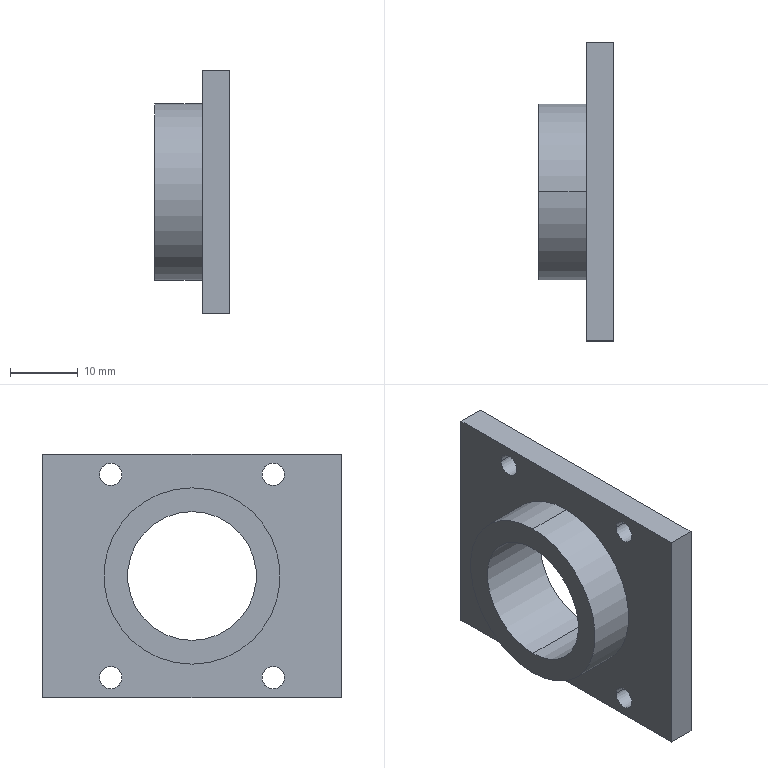Part | SolidWorks | features BaseBody 1 | 1 solid | 19 faces | box 11 x 44 x 36 mm | volume 6797 mm3 | cylinder 12 | plane 7 | commonest cylinder face diameters 3.3 x8 19 x2 26 x2
STEP:
#1=CARTESIAN_POINT('',(-2.,-13.65,33.));
#2=VERTEX_POINT('',#1);
#3=CARTESIAN_POINT('',(-2.,-10.35,33.));
#4=VERTEX_POINT('',#3);
#5=CARTESIAN_POINT('',(-2.,-12.,33.));
#6=DIRECTION('',(1.,0.,0.));
#7=DIRECTION('',(0.,1.,0.));
#8=AXIS2_PLACEMENT_3D('',#5,#6,#7);
#9=CIRCLE('',#8,1.65);
#10=EDGE_CURVE('',#2,#4,#9,.T.);
#11=ORIENTED_EDGE('',*,*,#10,.F.);
#12=CARTESIAN_POINT('',(2.,-13.65,33.));
#13=VERTEX_POINT('',#12);
#14=CARTESIAN_POINT('',(-14.2,-13.65,33.));
#15=DIRECTION('',(1.,0.,0.));
#16=VECTOR('',#15,1000.);
#17=LINE('',#14,#16);
#18=EDGE_CURVE('',#2,#13,#17,.T.);
#19=ORIENTED_EDGE('',*,*,#18,.T.);
#20=CARTESIAN_POINT('',(2.,-10.35,33.));
#21=VERTEX_POINT('',#20);
#22=CARTESIAN_POINT('',(2.,-12.,33.));
#23=DIRECTION('',(-1.,0.,0.));
#24=DIRECTION('',(0.,1.,0.));
#25=AXIS2_PLACEMENT_3D('',#22,#23,#24);
#26=CIRCLE('',#25,1.65);
#27=EDGE_CURVE('',#21,#13,#26,.T.);
#28=ORIENTED_EDGE('',*,*,#27,.F.);
#29=CARTESIAN_POINT('',(-14.2,-10.35,33.));
#30=DIRECTION('',(1.,0.,0.));
#31=VECTOR('',#30,1000.);
#32=LINE('',#29,#31);
#33=EDGE_CURVE('',#4,#21,#32,.T.);
#34=ORIENTED_EDGE('',*,*,#33,.F.);
#35=EDGE_LOOP('',(#11,#19,#28,#34));
#36=FACE_OUTER_BOUND('',#35,.T.);
#37=CARTESIAN_POINT('',(-14.2,-12.,33.));
#38=DIRECTION('',(1.,0.,0.));
#39=DIRECTION('',(0.,1.,0.));
#40=AXIS2_PLACEMENT_3D('',#37,#38,#39);
#41=CYLINDRICAL_SURFACE('',#40,1.65);
#42=ADVANCED_FACE('',(#36),#41,.F.);
#43=CARTESIAN_POINT('',(-2.,-13.65,3.));
#44=VERTEX_POINT('',#43);
#45=CARTESIAN_POINT('',(-2.,-10.35,3.));
#46=VERTEX_POINT('',#45);
#47=CARTESIAN_POINT('',(-2.,-12.,3.));
#48=DIRECTION('',(1.,0.,0.));
#49=DIRECTION('',(0.,1.,0.));
#50=AXIS2_PLACEMENT_3D('',#47,#48,#49);
#51=CIRCLE('',#50,1.65);
#52=EDGE_CURVE('',#44,#46,#51,.T.);
#53=ORIENTED_EDGE('',*,*,#52,.F.);
#54=CARTESIAN_POINT('',(2.,-13.65,3.));
#55=VERTEX_POINT('',#54);
#56=CARTESIAN_POINT('',(-14.2,-13.65,3.));
#57=DIRECTION('',(1.,0.,0.));
#58=VECTOR('',#57,1000.);
#59=LINE('',#56,#58);
#60=EDGE_CURVE('',#44,#55,#59,.T.);
#61=ORIENTED_EDGE('',*,*,#60,.T.);
#62=CARTESIAN_POINT('',(2.,-10.35,3.));
#63=VERTEX_POINT('',#62);
#64=CARTESIAN_POINT('',(2.,-12.,3.));
#65=DIRECTION('',(-1.,0.,0.));
#66=DIRECTION('',(0.,1.,0.));
#67=AXIS2_PLACEMENT_3D('',#64,#65,#66);
#68=CIRCLE('',#67,1.65);
#69=EDGE_CURVE('',#63,#55,#68,.T.);
#70=ORIENTED_EDGE('',*,*,#69,.F.);
#71=CARTESIAN_POINT('',(-14.2,-10.35,3.));
#72=DIRECTION('',(1.,0.,0.));
#73=VECTOR('',#72,1000.);
#74=LINE('',#71,#73);
#75=EDGE_CURVE('',#46,#63,#74,.T.);
#76=ORIENTED_EDGE('',*,*,#75,.F.);
#77=EDGE_LOOP('',(#53,#61,#70,#76));
#78=FACE_OUTER_BOUND('',#77,.T.);
#79=CARTESIAN_POINT('',(-14.2,-12.,3.));
#80=DIRECTION('',(1.,0.,0.));
#81=DIRECTION('',(0.,1.,0.));
#82=AXIS2_PLACEMENT_3D('',#79,#80,#81);
#83=CYLINDRICAL_SURFACE('',#82,1.65);
#84=ADVANCED_FACE('',(#78),#83,.F.);
#85=CARTESIAN_POINT('',(-9.,0.,27.5));
#86=VERTEX_POINT('',#85);
#87=CARTESIAN_POINT('',(-9.,0.,8.5));
#88=VERTEX_POINT('',#87);
#89=CARTESIAN_POINT('',(-9.,0.,18.));
#90=DIRECTION('',(1.,0.,0.));
#91=DIRECTION('',(0.,0.,-1.));
#92=AXIS2_PLACEMENT_3D('',#89,#90,#91);
#93=CIRCLE('',#92,9.5);
#94=EDGE_CURVE('',#86,#88,#93,.T.);
#95=ORIENTED_EDGE('',*,*,#94,.F.);
#96=CARTESIAN_POINT('',(2.,0.,27.5));
#97=VERTEX_POINT('',#96);
#98=CARTESIAN_POINT('',(-3.,0.,27.5));
#99=DIRECTION('',(1.,0.,0.));
#100=VECTOR('',#99,1000.);
#101=LINE('',#98,#100);
#102=EDGE_CURVE('',#86,#97,#101,.T.);
#103=ORIENTED_EDGE('',*,*,#102,.T.);
#104=CARTESIAN_POINT('',(2.,0.,8.5));
#105=VERTEX_POINT('',#104);
#106=CARTESIAN_POINT('',(2.,0.,18.));
#107=DIRECTION('',(-1.,0.,0.));
#108=DIRECTION('',(0.,0.,-1.));
#109=AXIS2_PLACEMENT_3D('',#106,#107,#108);
#110=CIRCLE('',#109,9.5);
#111=EDGE_CURVE('',#105,#97,#110,.T.);
#112=ORIENTED_EDGE('',*,*,#111,.F.);
#113=CARTESIAN_POINT('',(-3.,0.,8.5));
#114=DIRECTION('',(1.,0.,0.));
#115=VECTOR('',#114,1000.);
#116=LINE('',#113,#115);
#117=EDGE_CURVE('',#88,#105,#116,.T.);
#118=ORIENTED_EDGE('',*,*,#117,.F.);
#119=EDGE_LOOP('',(#95,#103,#112,#118));
#120=FACE_OUTER_BOUND('',#119,.T.);
#121=CARTESIAN_POINT('',(-3.,0.,18.));
#122=DIRECTION('',(1.,0.,0.));
#123=DIRECTION('',(0.,0.,-1.));
#124=AXIS2_PLACEMENT_3D('',#121,#122,#123);
#125=CYLINDRICAL_SURFACE('',#124,9.5);
#126=ADVANCED_FACE('',(#120),#125,.F.);
#127=CARTESIAN_POINT('',(-2.,10.35,33.));
#128=VERTEX_POINT('',#127);
#129=CARTESIAN_POINT('',(-2.,13.65,33.));
#130=VERTEX_POINT('',#129);
#131=CARTESIAN_POINT('',(-2.,12.,33.));
#132=DIRECTION('',(1.,0.,0.));
#133=DIRECTION('',(0.,1.,0.));
#134=AXIS2_PLACEMENT_3D('',#131,#132,#133);
#135=CIRCLE('',#134,1.65);
#136=EDGE_CURVE('',#128,#130,#135,.T.);
#137=ORIENTED_EDGE('',*,*,#136,.F.);
#138=CARTESIAN_POINT('',(2.,10.35,33.));
#139=VERTEX_POINT('',#138);
#140=CARTESIAN_POINT('',(-14.2,10.35,33.));
#141=DIRECTION('',(1.,0.,0.));
#142=VECTOR('',#141,1000.);
#143=LINE('',#140,#142);
#144=EDGE_CURVE('',#128,#139,#143,.T.);
#145=ORIENTED_EDGE('',*,*,#144,.T.);
#146=CARTESIAN_POINT('',(2.,13.65,33.));
#147=VERTEX_POINT('',#146);
#148=CARTESIAN_POINT('',(2.,12.,33.));
#149=DIRECTION('',(-1.,0.,0.));
#150=DIRECTION('',(0.,1.,0.));
#151=AXIS2_PLACEMENT_3D('',#148,#149,#150);
#152=CIRCLE('',#151,1.65);
#153=EDGE_CURVE('',#147,#139,#152,.T.);
#154=ORIENTED_EDGE('',*,*,#153,.F.);
#155=CARTESIAN_POINT('',(-14.2,13.65,33.));
#156=DIRECTION('',(1.,0.,0.));
#157=VECTOR('',#156,1000.);
#158=LINE('',#155,#157);
#159=EDGE_CURVE('',#130,#147,#158,.T.);
#160=ORIENTED_EDGE('',*,*,#159,.F.);
#161=EDGE_LOOP('',(#137,#145,#154,#160));
#162=FACE_OUTER_BOUND('',#161,.T.);
#163=CARTESIAN_POINT('',(-14.2,12.,33.));
#164=DIRECTION('',(1.,0.,0.));
#165=DIRECTION('',(0.,1.,0.));
#166=AXIS2_PLACEMENT_3D('',#163,#164,#165);
#167=CYLINDRICAL_SURFACE('',#166,1.65);
#168=ADVANCED_FACE('',(#162),#167,.F.);
#169=CARTESIAN_POINT('',(-2.,10.35,3.));
#170=VERTEX_POINT('',#169);
#171=CARTESIAN_POINT('',(-2.,13.65,3.));
#172=VERTEX_POINT('',#171);
#173=CARTESIAN_POINT('',(-2.,12.,3.));
#174=DIRECTION('',(1.,0.,0.));
#175=DIRECTION('',(0.,1.,0.));
#176=AXIS2_PLACEMENT_3D('',#173,#174,#175);
#177=CIRCLE('',#176,1.65);
#178=EDGE_CURVE('',#170,#172,#177,.T.);
#179=ORIENTED_EDGE('',*,*,#178,.F.);
#180=CARTESIAN_POINT('',(2.,10.35,3.));
#181=VERTEX_POINT('',#180);
#182=CARTESIAN_POINT('',(-14.2,10.35,3.));
#183=DIRECTION('',(1.,0.,0.));
#184=VECTOR('',#183,1000.);
#185=LINE('',#182,#184);
#186=EDGE_CURVE('',#170,#181,#185,.T.);
#187=ORIENTED_EDGE('',*,*,#186,.T.);
#188=CARTESIAN_POINT('',(2.,13.65,3.));
#189=VERTEX_POINT('',#188);
#190=CARTESIAN_POINT('',(2.,12.,3.));
#191=DIRECTION('',(-1.,0.,0.));
#192=DIRECTION('',(0.,1.,0.));
#193=AXIS2_PLACEMENT_3D('',#190,#191,#192);
#194=CIRCLE('',#193,1.65);
#195=EDGE_CURVE('',#189,#181,#194,.T.);
#196=ORIENTED_EDGE('',*,*,#195,.F.);
#197=CARTESIAN_POINT('',(-14.2,13.65,3.));
#198=DIRECTION('',(1.,0.,0.));
#199=VECTOR('',#198,1000.);
#200=LINE('',#197,#199);
#201=EDGE_CURVE('',#172,#189,#200,.T.);
#202=ORIENTED_EDGE('',*,*,#201,.F.);
#203=EDGE_LOOP('',(#179,#187,#196,#202));
#204=FACE_OUTER_BOUND('',#203,.T.);
#205=CARTESIAN_POINT('',(-14.2,12.,3.));
#206=DIRECTION('',(1.,0.,0.));
#207=DIRECTION('',(0.,1.,0.));
#208=AXIS2_PLACEMENT_3D('',#205,#206,#207);
#209=CYLINDRICAL_SURFACE('',#208,1.65);
#210=ADVANCED_FACE('',(#204),#209,.F.);
#211=CARTESIAN_POINT('',(-9.,0.,5.));
#212=VERTEX_POINT('',#211);
#213=CARTESIAN_POINT('',(-9.,0.,31.));
#214=VERTEX_POINT('',#213);
#215=CARTESIAN_POINT('',(-9.,0.,18.));
#216=DIRECTION('',(1.,0.,0.));
#217=DIRECTION('',(0.,0.,-1.));
#218=AXIS2_PLACEMENT_3D('',#215,#216,#217);
#219=CIRCLE('',#218,13.);
#220=EDGE_CURVE('',#212,#214,#219,.T.);
#221=ORIENTED_EDGE('',*,*,#220,.T.);
#222=CARTESIAN_POINT('',(-2.,0.,31.));
#223=VERTEX_POINT('',#222);
#224=CARTESIAN_POINT('',(-9.,0.,31.));
#225=DIRECTION('',(1.,0.,0.));
#226=VECTOR('',#225,1000.);
#227=LINE('',#224,#226);
#228=EDGE_CURVE('',#214,#223,#227,.T.);
#229=ORIENTED_EDGE('',*,*,#228,.T.);
#230=CARTESIAN_POINT('',(-2.,0.,5.));
#231=VERTEX_POINT('',#230);
#232=CARTESIAN_POINT('',(-2.,0.,18.));
#233=DIRECTION('',(-1.,0.,0.));
#234=DIRECTION('',(0.,0.,-1.));
#235=AXIS2_PLACEMENT_3D('',#232,#233,#234);
#236=CIRCLE('',#235,13.);
#237=EDGE_CURVE('',#223,#231,#236,.T.);
#238=ORIENTED_EDGE('',*,*,#237,.T.);
#239=CARTESIAN_POINT('',(-9.,0.,5.));
#240=DIRECTION('',(1.,0.,0.));
#241=VECTOR('',#240,1000.);
#242=LINE('',#239,#241);
#243=EDGE_CURVE('',#212,#231,#242,.T.);
#244=ORIENTED_EDGE('',*,*,#243,.F.);
#245=EDGE_LOOP('',(#221,#229,#238,#244));
#246=FACE_OUTER_BOUND('',#245,.T.);
#247=CARTESIAN_POINT('',(-9.,0.,18.));
#248=DIRECTION('',(1.,0.,0.));
#249=DIRECTION('',(0.,0.,-1.));
#250=AXIS2_PLACEMENT_3D('',#247,#248,#249);
#251=CYLINDRICAL_SURFACE('',#250,13.);
#252=ADVANCED_FACE('',(#246),#251,.T.);
#253=ORIENTED_EDGE('',*,*,#27,.T.);
#254=CARTESIAN_POINT('',(2.,-12.,33.));
#255=DIRECTION('',(-1.,0.,0.));
#256=DIRECTION('',(0.,1.,0.));
#257=AXIS2_PLACEMENT_3D('',#254,#255,#256);
#258=CIRCLE('',#257,1.65);
#259=EDGE_CURVE('',#13,#21,#258,.T.);
#260=ORIENTED_EDGE('',*,*,#259,.T.);
#261=EDGE_LOOP('',(#253,#260));
#262=FACE_BOUND('',#261,.T.);
#263=ORIENTED_EDGE('',*,*,#69,.T.);
#264=CARTESIAN_POINT('',(2.,-12.,3.));
#265=DIRECTION('',(-1.,0.,0.));
#266=DIRECTION('',(0.,1.,0.));
#267=AXIS2_PLACEMENT_3D('',#264,#265,#266);
#268=CIRCLE('',#267,1.65);
#269=EDGE_CURVE('',#55,#63,#268,.T.);
#270=ORIENTED_EDGE('',*,*,#269,.T.);
#271=EDGE_LOOP('',(#263,#270));
#272=FACE_BOUND('',#271,.T.);
#273=ORIENTED_EDGE('',*,*,#111,.T.);
#274=CARTESIAN_POINT('',(2.,0.,18.));
#275=DIRECTION('',(-1.,0.,0.));
#276=DIRECTION('',(0.,0.,-1.));
#277=AXIS2_PLACEMENT_3D('',#274,#275,#276);
#278=CIRCLE('',#277,9.5);
#279=EDGE_CURVE('',#97,#105,#278,.T.);
#280=ORIENTED_EDGE('',*,*,#279,.T.);
#281=EDGE_LOOP('',(#273,#280));
#282=FACE_BOUND('',#281,.T.);
#283=ORIENTED_EDGE('',*,*,#153,.T.);
#284=CARTESIAN_POINT('',(2.,12.,33.));
#285=DIRECTION('',(-1.,0.,0.));
#286=DIRECTION('',(0.,1.,0.));
#287=AXIS2_PLACEMENT_3D('',#284,#285,#286);
#288=CIRCLE('',#287,1.65);
#289=EDGE_CURVE('',#139,#147,#288,.T.);
#290=ORIENTED_EDGE('',*,*,#289,.T.);
#291=EDGE_LOOP('',(#283,#290));
#292=FACE_BOUND('',#291,.T.);
#293=ORIENTED_EDGE('',*,*,#195,.T.);
#294=CARTESIAN_POINT('',(2.,12.,3.));
#295=DIRECTION('',(-1.,0.,0.));
#296=DIRECTION('',(0.,1.,0.));
#297=AXIS2_PLACEMENT_3D('',#294,#295,#296);
#298=CIRCLE('',#297,1.65);
#299=EDGE_CURVE('',#181,#189,#298,.T.);
#300=ORIENTED_EDGE('',*,*,#299,.T.);
#301=EDGE_LOOP('',(#293,#300));
#302=FACE_BOUND('',#301,.T.);
#303=CARTESIAN_POINT('',(2.,22.,0.));
#304=VERTEX_POINT('',#303);
#305=CARTESIAN_POINT('',(2.,22.,36.));
#306=VERTEX_POINT('',#305);
#307=CARTESIAN_POINT('',(2.,22.,0.));
#308=DIRECTION('',(0.,0.,1.));
#309=VECTOR('',#308,1000.);
#310=LINE('',#307,#309);
#311=EDGE_CURVE('',#304,#306,#310,.T.);
#312=ORIENTED_EDGE('',*,*,#311,.T.);
#313=CARTESIAN_POINT('',(2.,-22.,36.));
#314=VERTEX_POINT('',#313);
#315=CARTESIAN_POINT('',(2.,-22.,36.));
#316=DIRECTION('',(0.,-1.,0.));
#317=VECTOR('',#316,1000.);
#318=LINE('',#315,#317);
#319=EDGE_CURVE('',#306,#314,#318,.T.);
#320=ORIENTED_EDGE('',*,*,#319,.T.);
#321=CARTESIAN_POINT('',(2.,-22.,0.));
#322=VERTEX_POINT('',#321);
#323=CARTESIAN_POINT('',(2.,-22.,0.));
#324=DIRECTION('',(0.,0.,-1.));
#325=VECTOR('',#324,1000.);
#326=LINE('',#323,#325);
#327=EDGE_CURVE('',#314,#322,#326,.T.);
#328=ORIENTED_EDGE('',*,*,#327,.T.);
#329=CARTESIAN_POINT('',(2.,-22.,0.));
#330=DIRECTION('',(0.,1.,0.));
#331=VECTOR('',#330,1000.);
#332=LINE('',#329,#331);
#333=EDGE_CURVE('',#322,#304,#332,.T.);
#334=ORIENTED_EDGE('',*,*,#333,.T.);
#335=EDGE_LOOP('',(#312,#320,#328,#334));
#336=FACE_OUTER_BOUND('',#335,.T.);
#337=CARTESIAN_POINT('',(2.,-22.,0.));
#338=DIRECTION('',(1.,0.,0.));
#339=DIRECTION('',(0.,0.,-1.));
#340=AXIS2_PLACEMENT_3D('',#337,#338,#339);
#341=PLANE('',#340);
#342=ADVANCED_FACE('',(#262,#272,#282,#292,#302,#336),#341,.T.);
#343=ORIENTED_EDGE('',*,*,#18,.F.);
#344=CARTESIAN_POINT('',(-2.,-12.,33.));
#345=DIRECTION('',(1.,0.,0.));
#346=DIRECTION('',(0.,1.,0.));
#347=AXIS2_PLACEMENT_3D('',#344,#345,#346);
#348=CIRCLE('',#347,1.65);
#349=EDGE_CURVE('',#4,#2,#348,.T.);
#350=ORIENTED_EDGE('',*,*,#349,.F.);
#351=ORIENTED_EDGE('',*,*,#33,.T.);
#352=ORIENTED_EDGE('',*,*,#259,.F.);
#353=EDGE_LOOP('',(#343,#350,#351,#352));
#354=FACE_OUTER_BOUND('',#353,.T.);
#355=CARTESIAN_POINT('',(-14.2,-12.,33.));
#356=DIRECTION('',(1.,0.,0.));
#357=DIRECTION('',(0.,1.,0.));
#358=AXIS2_PLACEMENT_3D('',#355,#356,#357);
#359=CYLINDRICAL_SURFACE('',#358,1.65);
#360=ADVANCED_FACE('',(#354),#359,.F.);
#361=ORIENTED_EDGE('',*,*,#60,.F.);
#362=CARTESIAN_POINT('',(-2.,-12.,3.));
#363=DIRECTION('',(1.,0.,0.));
#364=DIRECTION('',(0.,1.,0.));
#365=AXIS2_PLACEMENT_3D('',#362,#363,#364);
#366=CIRCLE('',#365,1.65);
#367=EDGE_CURVE('',#46,#44,#366,.T.);
#368=ORIENTED_EDGE('',*,*,#367,.F.);
#369=ORIENTED_EDGE('',*,*,#75,.T.);
#370=ORIENTED_EDGE('',*,*,#269,.F.);
#371=EDGE_LOOP('',(#361,#368,#369,#370));
#372=FACE_OUTER_BOUND('',#371,.T.);
#373=CARTESIAN_POINT('',(-14.2,-12.,3.));
#374=DIRECTION('',(1.,0.,0.));
#375=DIRECTION('',(0.,1.,0.));
#376=AXIS2_PLACEMENT_3D('',#373,#374,#375);
#377=CYLINDRICAL_SURFACE('',#376,1.65);
#378=ADVANCED_FACE('',(#372),#377,.F.);
#379=ORIENTED_EDGE('',*,*,#102,.F.);
#380=CARTESIAN_POINT('',(-9.,0.,18.));
#381=DIRECTION('',(1.,0.,0.));
#382=DIRECTION('',(0.,0.,-1.));
#383=AXIS2_PLACEMENT_3D('',#380,#381,#382);
#384=CIRCLE('',#383,9.5);
#385=EDGE_CURVE('',#88,#86,#384,.T.);
#386=ORIENTED_EDGE('',*,*,#385,.F.);
#387=ORIENTED_EDGE('',*,*,#117,.T.);
#388=ORIENTED_EDGE('',*,*,#279,.F.);
#389=EDGE_LOOP('',(#379,#386,#387,#388));
#390=FACE_OUTER_BOUND('',#389,.T.);
#391=CARTESIAN_POINT('',(-3.,0.,18.));
#392=DIRECTION('',(1.,0.,0.));
#393=DIRECTION('',(0.,0.,-1.));
#394=AXIS2_PLACEMENT_3D('',#391,#392,#393);
#395=CYLINDRICAL_SURFACE('',#394,9.5);
#396=ADVANCED_FACE('',(#390),#395,.F.);
#397=ORIENTED_EDGE('',*,*,#144,.F.);
#398=CARTESIAN_POINT('',(-2.,12.,33.));
#399=DIRECTION('',(1.,0.,0.));
#400=DIRECTION('',(0.,1.,0.));
#401=AXIS2_PLACEMENT_3D('',#398,#399,#400);
#402=CIRCLE('',#401,1.65);
#403=EDGE_CURVE('',#130,#128,#402,.T.);
#404=ORIENTED_EDGE('',*,*,#403,.F.);
#405=ORIENTED_EDGE('',*,*,#159,.T.);
#406=ORIENTED_EDGE('',*,*,#289,.F.);
#407=EDGE_LOOP('',(#397,#404,#405,#406));
#408=FACE_OUTER_BOUND('',#407,.T.);
#409=CARTESIAN_POINT('',(-14.2,12.,33.));
#410=DIRECTION('',(1.,0.,0.));
#411=DIRECTION('',(0.,1.,0.));
#412=AXIS2_PLACEMENT_3D('',#409,#410,#411);
#413=CYLINDRICAL_SURFACE('',#412,1.65);
#414=ADVANCED_FACE('',(#408),#413,.F.);
#415=ORIENTED_EDGE('',*,*,#186,.F.);
#416=CARTESIAN_POINT('',(-2.,12.,3.));
#417=DIRECTION('',(1.,0.,0.));
#418=DIRECTION('',(0.,1.,0.));
#419=AXIS2_PLACEMENT_3D('',#416,#417,#418);
#420=CIRCLE('',#419,1.65);
#421=EDGE_CURVE('',#172,#170,#420,.T.);
#422=ORIENTED_EDGE('',*,*,#421,.F.);
#423=ORIENTED_EDGE('',*,*,#201,.T.);
#424=ORIENTED_EDGE('',*,*,#299,.F.);
#425=EDGE_LOOP('',(#415,#422,#423,#424));
#426=FACE_OUTER_BOUND('',#425,.T.);
#427=CARTESIAN_POINT('',(-14.2,12.,3.));
#428=DIRECTION('',(1.,0.,0.));
#429=DIRECTION('',(0.,1.,0.));
#430=AXIS2_PLACEMENT_3D('',#427,#428,#429);
#431=CYLINDRICAL_SURFACE('',#430,1.65);
#432=ADVANCED_FACE('',(#426),#431,.F.);
#433=ORIENTED_EDGE('',*,*,#319,.F.);
#434=CARTESIAN_POINT('',(-2.,22.,36.));
#435=VERTEX_POINT('',#434);
#436=CARTESIAN_POINT('',(-2.,22.,36.));
#437=DIRECTION('',(-1.,0.,0.));
#438=VECTOR('',#437,1000.);
#439=LINE('',#436,#438);
#440=EDGE_CURVE('',#306,#435,#439,.T.);
#441=ORIENTED_EDGE('',*,*,#440,.T.);
#442=CARTESIAN_POINT('',(-2.,-22.,36.));
#443=VERTEX_POINT('',#442);
#444=CARTESIAN_POINT('',(-2.,-22.,36.));
#445=DIRECTION('',(0.,-1.,0.));
#446=VECTOR('',#445,1000.);
#447=LINE('',#444,#446);
#448=EDGE_CURVE('',#435,#443,#447,.T.);
#449=ORIENTED_EDGE('',*,*,#448,.T.);
#450=CARTESIAN_POINT('',(-2.,-22.,36.));
#451=DIRECTION('',(1.,0.,0.));
#452=VECTOR('',#451,1000.);
#453=LINE('',#450,#452);
#454=EDGE_CURVE('',#443,#314,#453,.T.);
#455=ORIENTED_EDGE('',*,*,#454,.T.);
#456=EDGE_LOOP('',(#433,#441,#449,#455));
#457=FACE_OUTER_BOUND('',#456,.T.);
#458=CARTESIAN_POINT('',(-2.,-22.,36.));
#459=DIRECTION('',(0.,0.,1.));
#460=DIRECTION('',(1.,0.,0.));
#461=AXIS2_PLACEMENT_3D('',#458,#459,#460);
#462=PLANE('',#461);
#463=ADVANCED_FACE('',(#457),#462,.T.);
#464=ORIENTED_EDGE('',*,*,#440,.F.);
#465=ORIENTED_EDGE('',*,*,#311,.F.);
#466=CARTESIAN_POINT('',(-2.,22.,0.));
#467=VERTEX_POINT('',#466);
#468=CARTESIAN_POINT('',(-2.,22.,0.));
#469=DIRECTION('',(-1.,0.,0.));
#470=VECTOR('',#469,1000.);
#471=LINE('',#468,#470);
#472=EDGE_CURVE('',#304,#467,#471,.T.);
#473=ORIENTED_EDGE('',*,*,#472,.T.);
#474=CARTESIAN_POINT('',(-2.,22.,0.));
#475=DIRECTION('',(0.,0.,1.));
#476=VECTOR('',#475,1000.);
#477=LINE('',#474,#476);
#478=EDGE_CURVE('',#467,#435,#477,.T.);
#479=ORIENTED_EDGE('',*,*,#478,.T.);
#480=EDGE_LOOP('',(#464,#465,#473,#479));
#481=FACE_OUTER_BOUND('',#480,.T.);
#482=CARTESIAN_POINT('',(-2.,22.,0.));
#483=DIRECTION('',(0.,1.,0.));
#484=DIRECTION('',(0.,0.,1.));
#485=AXIS2_PLACEMENT_3D('',#482,#483,#484);
#486=PLANE('',#485);
#487=ADVANCED_FACE('',(#481),#486,.T.);
#488=ORIENTED_EDGE('',*,*,#333,.F.);
#489=CARTESIAN_POINT('',(-2.,-22.,0.));
#490=VERTEX_POINT('',#489);
#491=CARTESIAN_POINT('',(-2.,-22.,0.));
#492=DIRECTION('',(1.,0.,0.));
#493=VECTOR('',#492,1000.);
#494=LINE('',#491,#493);
#495=EDGE_CURVE('',#490,#322,#494,.T.);
#496=ORIENTED_EDGE('',*,*,#495,.F.);
#497=CARTESIAN_POINT('',(-2.,-22.,0.));
#498=DIRECTION('',(0.,-1.,0.));
#499=VECTOR('',#498,1000.);
#500=LINE('',#497,#499);
#501=EDGE_CURVE('',#467,#490,#500,.T.);
#502=ORIENTED_EDGE('',*,*,#501,.F.);
#503=ORIENTED_EDGE('',*,*,#472,.F.);
#504=EDGE_LOOP('',(#488,#496,#502,#503));
#505=FACE_OUTER_BOUND('',#504,.T.);
#506=CARTESIAN_POINT('',(-2.,-22.,0.));
#507=DIRECTION('',(0.,0.,1.));
#508=DIRECTION('',(1.,0.,0.));
#509=AXIS2_PLACEMENT_3D('',#506,#507,#508);
#510=PLANE('',#509);
#511=ADVANCED_FACE('',(#505),#510,.F.);
#512=ORIENTED_EDGE('',*,*,#454,.F.);
#513=CARTESIAN_POINT('',(-2.,-22.,0.));
#514=DIRECTION('',(0.,0.,1.));
#515=VECTOR('',#514,1000.);
#516=LINE('',#513,#515);
#517=EDGE_CURVE('',#490,#443,#516,.T.);
#518=ORIENTED_EDGE('',*,*,#517,.F.);
#519=ORIENTED_EDGE('',*,*,#495,.T.);
#520=ORIENTED_EDGE('',*,*,#327,.F.);
#521=EDGE_LOOP('',(#512,#518,#519,#520));
#522=FACE_OUTER_BOUND('',#521,.T.);
#523=CARTESIAN_POINT('',(-2.,-22.,0.));
#524=DIRECTION('',(0.,1.,0.));
#525=DIRECTION('',(0.,0.,1.));
#526=AXIS2_PLACEMENT_3D('',#523,#524,#525);
#527=PLANE('',#526);
#528=ADVANCED_FACE('',(#522),#527,.F.);
#529=ORIENTED_EDGE('',*,*,#349,.T.);
#530=ORIENTED_EDGE('',*,*,#10,.T.);
#531=EDGE_LOOP('',(#529,#530));
#532=FACE_BOUND('',#531,.T.);
#533=ORIENTED_EDGE('',*,*,#367,.T.);
#534=ORIENTED_EDGE('',*,*,#52,.T.);
#535=EDGE_LOOP('',(#533,#534));
#536=FACE_BOUND('',#535,.T.);
#537=CARTESIAN_POINT('',(-2.,0.,18.));
#538=DIRECTION('',(-1.,0.,0.));
#539=DIRECTION('',(0.,0.,-1.));
#540=AXIS2_PLACEMENT_3D('',#537,#538,#539);
#541=CIRCLE('',#540,13.);
#542=EDGE_CURVE('',#231,#223,#541,.T.);
#543=ORIENTED_EDGE('',*,*,#542,.F.);
#544=ORIENTED_EDGE('',*,*,#237,.F.);
#545=EDGE_LOOP('',(#543,#544));
#546=FACE_BOUND('',#545,.T.);
#547=ORIENTED_EDGE('',*,*,#403,.T.);
#548=ORIENTED_EDGE('',*,*,#136,.T.);
#549=EDGE_LOOP('',(#547,#548));
#550=FACE_BOUND('',#549,.T.);
#551=ORIENTED_EDGE('',*,*,#421,.T.);
#552=ORIENTED_EDGE('',*,*,#178,.T.);
#553=EDGE_LOOP('',(#551,#552));
#554=FACE_BOUND('',#553,.T.);
#555=ORIENTED_EDGE('',*,*,#478,.F.);
#556=ORIENTED_EDGE('',*,*,#501,.T.);
#557=ORIENTED_EDGE('',*,*,#517,.T.);
#558=ORIENTED_EDGE('',*,*,#448,.F.);
#559=EDGE_LOOP('',(#555,#556,#557,#558));
#560=FACE_OUTER_BOUND('',#559,.T.);
#561=CARTESIAN_POINT('',(-2.,-22.,0.));
#562=DIRECTION('',(1.,0.,0.));
#563=DIRECTION('',(0.,0.,-1.));
#564=AXIS2_PLACEMENT_3D('',#561,#562,#563);
#565=PLANE('',#564);
#566=ADVANCED_FACE('',(#532,#536,#546,#550,#554,#560),#565,.F.);
#567=ORIENTED_EDGE('',*,*,#385,.T.);
#568=ORIENTED_EDGE('',*,*,#94,.T.);
#569=EDGE_LOOP('',(#567,#568));
#570=FACE_BOUND('',#569,.T.);
#571=ORIENTED_EDGE('',*,*,#220,.F.);
#572=CARTESIAN_POINT('',(-9.,0.,18.));
#573=DIRECTION('',(1.,0.,0.));
#574=DIRECTION('',(0.,0.,-1.));
#575=AXIS2_PLACEMENT_3D('',#572,#573,#574);
#576=CIRCLE('',#575,13.);
#577=EDGE_CURVE('',#214,#212,#576,.T.);
#578=ORIENTED_EDGE('',*,*,#577,.F.);
#579=EDGE_LOOP('',(#571,#578));
#580=FACE_OUTER_BOUND('',#579,.T.);
#581=CARTESIAN_POINT('',(-9.,0.,18.));
#582=DIRECTION('',(1.,0.,0.));
#583=DIRECTION('',(0.,0.,-1.));
#584=AXIS2_PLACEMENT_3D('',#581,#582,#583);
#585=PLANE('',#584);
#586=ADVANCED_FACE('',(#570,#580),#585,.F.);
#587=ORIENTED_EDGE('',*,*,#228,.F.);
#588=ORIENTED_EDGE('',*,*,#577,.T.);
#589=ORIENTED_EDGE('',*,*,#243,.T.);
#590=ORIENTED_EDGE('',*,*,#542,.T.);
#591=EDGE_LOOP('',(#587,#588,#589,#590));
#592=FACE_OUTER_BOUND('',#591,.T.);
#593=CARTESIAN_POINT('',(-9.,0.,18.));
#594=DIRECTION('',(1.,0.,0.));
#595=DIRECTION('',(0.,0.,-1.));
#596=AXIS2_PLACEMENT_3D('',#593,#594,#595);
#597=CYLINDRICAL_SURFACE('',#596,13.);
#598=ADVANCED_FACE('',(#592),#597,.T.);
#599=CLOSED_SHELL('',(#42,#84,#126,#168,#210,#252,#342,#360,#378,#396,#414,#432,#463,#487,#511,#528,#566,#586,#598));
#600=MANIFOLD_SOLID_BREP('',#599);
#601=CARTESIAN_POINT('',(0.,0.,0.));
#602=DIRECTION('',(0.,0.,1.));
#603=DIRECTION('',(1.,0.,0.));
#604=AXIS2_PLACEMENT_3D('',#601,#602,#603);
#605=(LENGTH_UNIT()NAMED_UNIT(*)SI_UNIT(.MILLI.,.METRE.));
#606=UNCERTAINTY_MEASURE_WITH_UNIT(LENGTH_MEASURE(0.00001),#605,'','');
#607=(NAMED_UNIT(*)PLANE_ANGLE_UNIT()SI_UNIT($,.RADIAN.));
#608=(NAMED_UNIT(*)SI_UNIT($,.STERADIAN.)SOLID_ANGLE_UNIT());
#609=(GEOMETRIC_REPRESENTATION_CONTEXT(3)GLOBAL_UNCERTAINTY_ASSIGNED_CONTEXT((#606))GLOBAL_UNIT_ASSIGNED_CONTEXT((#605,#607,#608))REPRESENTATION_CONTEXT('',''));
#610=ADVANCED_BREP_SHAPE_REPRESENTATION('',(#600,#604),#609);